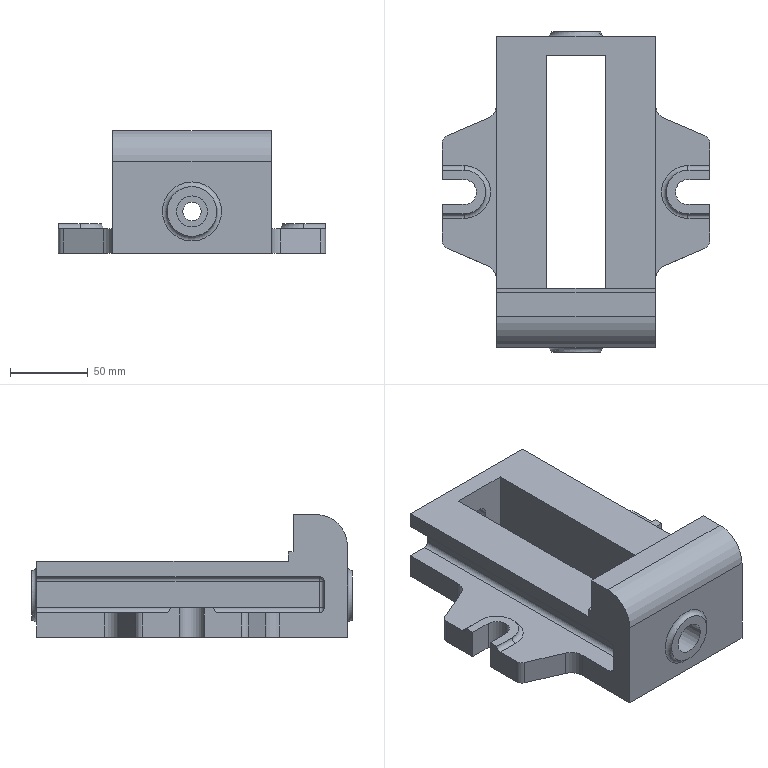Part | NX | features EXTRUDE 13, BLEND 11, DATUM_CSYS 10, SKETCH 9, EXTRACT_STRING 8, Instance Feature 2, Mirror Feature 2, SIMPLE HOLE 2, SYMBOLIC_THREAD 2, HOLE PACKAGE 1 | 1 solid | 82 faces | box 172 x 206 x 79 mm | volume 739526 mm3 | plane 43 | cylinder 29 | sphere 4 | torus 4 | cone 2 | commonest cylinder face diameters 6 x14 20 x5 10 x4 5 x2 16 x2 12 x1